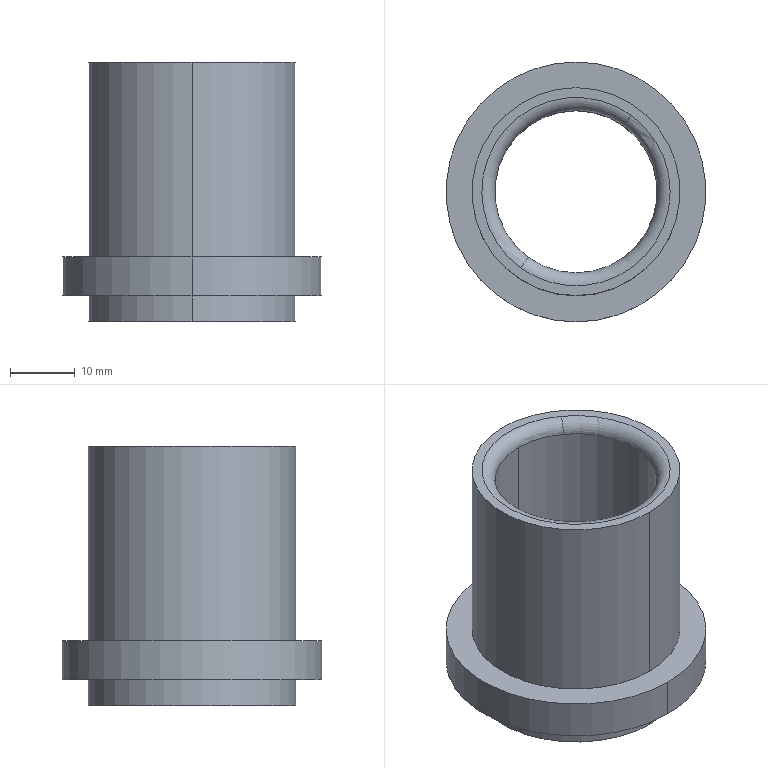Part | 1 solid | 16 faces | box 40 x 40 x 40 mm | volume 15162 mm3 | cylinder 8 | plane 4 | torus 4 | commonest cylinder face diameters 32 x4 25 x2 40 x2
STEP:
#1=CARTESIAN_POINT('',(0.,0.,0.));
#2=DIRECTION('',(0.,0.,1.));
#3=DIRECTION('',(1.,0.,0.));
#4=AXIS2_PLACEMENT_3D('',#1,#2,#3);
#5=CARTESIAN_POINT('',(-335.,26.5,-133.051));
#6=VERTEX_POINT('',#5);
#7=CARTESIAN_POINT('',(-335.,58.5,-133.051));
#8=VERTEX_POINT('',#7);
#9=CARTESIAN_POINT('',(-335.,42.5,-133.051));
#10=DIRECTION('',(0.,0.,1.));
#11=DIRECTION('',(0.,1.,0.));
#12=AXIS2_PLACEMENT_3D('',#9,#10,#11);
#13=CIRCLE('',#12,16.);
#14=CARTESIAN_POINT('',(-319.,42.5,-133.051));
#15=DIRECTION('',(0.,0.,-1.));
#16=DIRECTION('',(0.,-1.,0.));
#17=AXIS2_PLACEMENT_3D('',#14,#15,#16);
#18=PLANE('',#17);
#19=CARTESIAN_POINT('',(-16.,16.));
#20=CARTESIAN_POINT('',(-16.,43.713));
#21=CARTESIAN_POINT('',(8.,29.856));
#22=CARTESIAN_POINT('',(32.,16.));
#23=CARTESIAN_POINT('',(8.,2.144));
#24=CARTESIAN_POINT('',(-16.,-11.713));
#25=CARTESIAN_POINT('',(-16.,16.));
#26=(BOUNDED_CURVE()B_SPLINE_CURVE(2,(#19,#20,#21,#22,#23,#24,#25),.UNSPECIFIED.,.T.,.F.)B_SPLINE_CURVE_WITH_KNOTS((1,2,2,2,2,1),(-2.094,0.,2.094,4.189,6.283,8.378),.UNSPECIFIED.)CURVE()GEOMETRIC_REPRESENTATION_ITEM()RATIONAL_B_SPLINE_CURVE((1.,0.5,1.,0.5,1.,0.5,1.))REPRESENTATION_ITEM(''));
#27=(GEOMETRIC_REPRESENTATION_CONTEXT(2)PARAMETRIC_REPRESENTATION_CONTEXT()REPRESENTATION_CONTEXT('',''));
#28=DEFINITIONAL_REPRESENTATION('',(#26),#27);
#29=PCURVE('',#18,#28);
#30=CARTESIAN_POINT('',(-335.,42.5,-90.819));
#31=DIRECTION('',(0.,0.,1.));
#32=DIRECTION('',(-1.,0.,0.));
#33=AXIS2_PLACEMENT_3D('',#30,#31,#32);
#34=CYLINDRICAL_SURFACE('',#33,16.);
#35=CARTESIAN_POINT('',(-1.571,-42.232));
#36=DIRECTION('',(1.,0.));
#37=VECTOR('',#36,1.);
#38=LINE('',#35,#37);
#39=(GEOMETRIC_REPRESENTATION_CONTEXT(2)PARAMETRIC_REPRESENTATION_CONTEXT()REPRESENTATION_CONTEXT('',''));
#40=DEFINITIONAL_REPRESENTATION('',(#38),#39);
#41=PCURVE('',#34,#40);
#42=SURFACE_CURVE('',#13,(#29,#41),.PCURVE_S1.);
#43=EDGE_CURVE('',#6,#8,#42,.T.);
#44=ORIENTED_EDGE('',*,*,#43,.F.);
#45=CARTESIAN_POINT('',(-335.,42.5,-133.051));
#46=DIRECTION('',(0.,0.,1.));
#47=DIRECTION('',(0.,1.,0.));
#48=AXIS2_PLACEMENT_3D('',#45,#46,#47);
#49=CIRCLE('',#48,16.);
#50=CARTESIAN_POINT('',(-16.,16.));
#51=CARTESIAN_POINT('',(-16.,43.713));
#52=CARTESIAN_POINT('',(8.,29.856));
#53=CARTESIAN_POINT('',(32.,16.));
#54=CARTESIAN_POINT('',(8.,2.144));
#55=CARTESIAN_POINT('',(-16.,-11.713));
#56=CARTESIAN_POINT('',(-16.,16.));
#57=(BOUNDED_CURVE()B_SPLINE_CURVE(2,(#50,#51,#52,#53,#54,#55,#56),.UNSPECIFIED.,.T.,.F.)B_SPLINE_CURVE_WITH_KNOTS((1,2,2,2,2,1),(-2.094,0.,2.094,4.189,6.283,8.378),.UNSPECIFIED.)CURVE()GEOMETRIC_REPRESENTATION_ITEM()RATIONAL_B_SPLINE_CURVE((1.,0.5,1.,0.5,1.,0.5,1.))REPRESENTATION_ITEM(''));
#58=(GEOMETRIC_REPRESENTATION_CONTEXT(2)PARAMETRIC_REPRESENTATION_CONTEXT()REPRESENTATION_CONTEXT('',''));
#59=DEFINITIONAL_REPRESENTATION('',(#57),#58);
#60=PCURVE('',#18,#59);
#61=CARTESIAN_POINT('',(-335.,42.5,-90.819));
#62=DIRECTION('',(0.,0.,1.));
#63=DIRECTION('',(1.,0.,0.));
#64=AXIS2_PLACEMENT_3D('',#61,#62,#63);
#65=CYLINDRICAL_SURFACE('',#64,16.);
#66=CARTESIAN_POINT('',(1.571,-42.232));
#67=DIRECTION('',(1.,0.));
#68=VECTOR('',#67,1.);
#69=LINE('',#66,#68);
#70=(GEOMETRIC_REPRESENTATION_CONTEXT(2)PARAMETRIC_REPRESENTATION_CONTEXT()REPRESENTATION_CONTEXT('',''));
#71=DEFINITIONAL_REPRESENTATION('',(#69),#70);
#72=PCURVE('',#65,#71);
#73=SURFACE_CURVE('',#49,(#60,#72),.PCURVE_S1.);
#74=EDGE_CURVE('',#8,#6,#73,.T.);
#75=ORIENTED_EDGE('',*,*,#74,.F.);
#76=EDGE_LOOP('',(#44,#75));
#77=FACE_BOUND('',#76,.T.);
#78=CARTESIAN_POINT('',(-327.065,31.578,-133.051));
#79=VERTEX_POINT('',#78);
#80=CARTESIAN_POINT('',(-327.065,53.422,-133.051));
#81=VERTEX_POINT('',#80);
#82=CARTESIAN_POINT('',(-335.,42.5,-133.051));
#83=DIRECTION('',(0.,0.,1.));
#84=DIRECTION('',(0.5878,-0.809,0.));
#85=AXIS2_PLACEMENT_3D('',#82,#83,#84);
#86=CIRCLE('',#85,13.5);
#87=CARTESIAN_POINT('',(10.922,8.065));
#88=CARTESIAN_POINT('',(-2.822,-10.852));
#89=CARTESIAN_POINT('',(-12.333,10.509));
#90=CARTESIAN_POINT('',(-21.843,31.87));
#91=CARTESIAN_POINT('',(1.411,29.426));
#92=CARTESIAN_POINT('',(24.666,26.982));
#93=CARTESIAN_POINT('',(10.922,8.065));
#94=(BOUNDED_CURVE()B_SPLINE_CURVE(2,(#87,#88,#89,#90,#91,#92,#93),.UNSPECIFIED.,.T.,.F.)B_SPLINE_CURVE_WITH_KNOTS((1,2,2,2,2,1),(-2.094,0.,2.094,4.189,6.283,8.378),.UNSPECIFIED.)CURVE()GEOMETRIC_REPRESENTATION_ITEM()RATIONAL_B_SPLINE_CURVE((1.,0.5,1.,0.5,1.,0.5,1.))REPRESENTATION_ITEM(''));
#95=(GEOMETRIC_REPRESENTATION_CONTEXT(2)PARAMETRIC_REPRESENTATION_CONTEXT()REPRESENTATION_CONTEXT('',''));
#96=DEFINITIONAL_REPRESENTATION('',(#94),#95);
#97=PCURVE('',#18,#96);
#98=CARTESIAN_POINT('',(-335.,42.5,-132.051));
#99=DIRECTION('',(0.,0.,1.));
#100=DIRECTION('',(-0.809,0.5878,0.));
#101=AXIS2_PLACEMENT_3D('',#98,#99,#100);
#102=TOROIDAL_SURFACE('',#101,13.5,1.);
#103=CARTESIAN_POINT('',(2.827,4.712));
#104=DIRECTION('',(1.,0.));
#105=VECTOR('',#104,1.);
#106=LINE('',#103,#105);
#107=(GEOMETRIC_REPRESENTATION_CONTEXT(2)PARAMETRIC_REPRESENTATION_CONTEXT()REPRESENTATION_CONTEXT('',''));
#108=DEFINITIONAL_REPRESENTATION('',(#106),#107);
#109=PCURVE('',#102,#108);
#110=SURFACE_CURVE('',#86,(#97,#109),.PCURVE_S1.);
#111=EDGE_CURVE('',#79,#81,#110,.T.);
#112=ORIENTED_EDGE('',*,*,#111,.T.);
#113=CARTESIAN_POINT('',(-342.935,31.578,-133.051));
#114=VERTEX_POINT('',#113);
#115=CARTESIAN_POINT('',(-335.,42.5,-133.051));
#116=DIRECTION('',(0.,0.,1.));
#117=DIRECTION('',(0.5878,-0.809,0.));
#118=AXIS2_PLACEMENT_3D('',#115,#116,#117);
#119=CIRCLE('',#118,13.5);
#120=CARTESIAN_POINT('',(10.922,8.065));
#121=CARTESIAN_POINT('',(-2.822,-10.852));
#122=CARTESIAN_POINT('',(-12.333,10.509));
#123=CARTESIAN_POINT('',(-21.843,31.87));
#124=CARTESIAN_POINT('',(1.411,29.426));
#125=CARTESIAN_POINT('',(24.666,26.982));
#126=CARTESIAN_POINT('',(10.922,8.065));
#127=(BOUNDED_CURVE()B_SPLINE_CURVE(2,(#120,#121,#122,#123,#124,#125,#126),.UNSPECIFIED.,.T.,.F.)B_SPLINE_CURVE_WITH_KNOTS((1,2,2,2,2,1),(-2.094,0.,2.094,4.189,6.283,8.378),.UNSPECIFIED.)CURVE()GEOMETRIC_REPRESENTATION_ITEM()RATIONAL_B_SPLINE_CURVE((1.,0.5,1.,0.5,1.,0.5,1.))REPRESENTATION_ITEM(''));
#128=(GEOMETRIC_REPRESENTATION_CONTEXT(2)PARAMETRIC_REPRESENTATION_CONTEXT()REPRESENTATION_CONTEXT('',''));
#129=DEFINITIONAL_REPRESENTATION('',(#127),#128);
#130=PCURVE('',#18,#129);
#131=CARTESIAN_POINT('',(-335.,42.5,-132.051));
#132=DIRECTION('',(0.,0.,1.));
#133=DIRECTION('',(0.809,-0.5878,0.));
#134=AXIS2_PLACEMENT_3D('',#131,#132,#133);
#135=TOROIDAL_SURFACE('',#134,13.5,1.);
#136=CARTESIAN_POINT('',(-0.3142,4.712));
#137=DIRECTION('',(1.,0.));
#138=VECTOR('',#137,1.);
#139=LINE('',#136,#138);
#140=(GEOMETRIC_REPRESENTATION_CONTEXT(2)PARAMETRIC_REPRESENTATION_CONTEXT()REPRESENTATION_CONTEXT('',''));
#141=DEFINITIONAL_REPRESENTATION('',(#139),#140);
#142=PCURVE('',#135,#141);
#143=SURFACE_CURVE('',#119,(#130,#142),.PCURVE_S1.);
#144=EDGE_CURVE('',#81,#114,#143,.T.);
#145=ORIENTED_EDGE('',*,*,#144,.T.);
#146=CARTESIAN_POINT('',(-335.,42.5,-133.051));
#147=DIRECTION('',(0.,0.,1.));
#148=DIRECTION('',(0.5878,-0.809,0.));
#149=AXIS2_PLACEMENT_3D('',#146,#147,#148);
#150=CIRCLE('',#149,13.5);
#151=CARTESIAN_POINT('',(10.922,8.065));
#152=CARTESIAN_POINT('',(-2.822,-10.852));
#153=CARTESIAN_POINT('',(-12.333,10.509));
#154=CARTESIAN_POINT('',(-21.843,31.87));
#155=CARTESIAN_POINT('',(1.411,29.426));
#156=CARTESIAN_POINT('',(24.666,26.982));
#157=CARTESIAN_POINT('',(10.922,8.065));
#158=(BOUNDED_CURVE()B_SPLINE_CURVE(2,(#151,#152,#153,#154,#155,#156,#157),.UNSPECIFIED.,.T.,.F.)B_SPLINE_CURVE_WITH_KNOTS((1,2,2,2,2,1),(-2.094,0.,2.094,4.189,6.283,8.378),.UNSPECIFIED.)CURVE()GEOMETRIC_REPRESENTATION_ITEM()RATIONAL_B_SPLINE_CURVE((1.,0.5,1.,0.5,1.,0.5,1.))REPRESENTATION_ITEM(''));
#159=(GEOMETRIC_REPRESENTATION_CONTEXT(2)PARAMETRIC_REPRESENTATION_CONTEXT()REPRESENTATION_CONTEXT('',''));
#160=DEFINITIONAL_REPRESENTATION('',(#158),#159);
#161=PCURVE('',#18,#160);
#162=CARTESIAN_POINT('',(-3.456,4.712));
#163=DIRECTION('',(1.,0.));
#164=VECTOR('',#163,1.);
#165=LINE('',#162,#164);
#166=(GEOMETRIC_REPRESENTATION_CONTEXT(2)PARAMETRIC_REPRESENTATION_CONTEXT()REPRESENTATION_CONTEXT('',''));
#167=DEFINITIONAL_REPRESENTATION('',(#165),#166);
#168=PCURVE('',#102,#167);
#169=SURFACE_CURVE('',#150,(#161,#168),.PCURVE_S1.);
#170=EDGE_CURVE('',#114,#79,#169,.T.);
#171=ORIENTED_EDGE('',*,*,#170,.T.);
#172=EDGE_LOOP('',(#112,#145,#171));
#173=FACE_BOUND('',#172,.T.);
#174=ADVANCED_FACE('',(#77,#173),#18,.T.);
#175=CARTESIAN_POINT('',(-342.347,32.387,-132.051));
#176=VERTEX_POINT('',#175);
#177=CARTESIAN_POINT('',(-342.935,31.578,-132.051));
#178=DIRECTION('',(0.809,-0.5878,0.));
#179=DIRECTION('',(0.,0.,-1.));
#180=AXIS2_PLACEMENT_3D('',#177,#178,#179);
#181=CIRCLE('',#180,1.);
#182=CARTESIAN_POINT('',(1.571,4.712));
#183=DIRECTION('',(0.,-1.));
#184=VECTOR('',#183,1.);
#185=LINE('',#182,#184);
#186=(GEOMETRIC_REPRESENTATION_CONTEXT(2)PARAMETRIC_REPRESENTATION_CONTEXT()REPRESENTATION_CONTEXT('',''));
#187=DEFINITIONAL_REPRESENTATION('',(#185),#186);
#188=PCURVE('',#102,#187);
#189=CARTESIAN_POINT('',(4.712,4.712));
#190=DIRECTION('',(0.,-1.));
#191=VECTOR('',#190,1.);
#192=LINE('',#189,#191);
#193=(GEOMETRIC_REPRESENTATION_CONTEXT(2)PARAMETRIC_REPRESENTATION_CONTEXT()REPRESENTATION_CONTEXT('',''));
#194=DEFINITIONAL_REPRESENTATION('',(#192),#193);
#195=PCURVE('',#135,#194);
#196=SURFACE_CURVE('',#181,(#188,#195),.PCURVE_S1.);
#197=EDGE_CURVE('',#114,#176,#196,.T.);
#198=ORIENTED_EDGE('',*,*,#197,.T.);
#199=CARTESIAN_POINT('',(-335.,30.,-132.051));
#200=VERTEX_POINT('',#199);
#201=CARTESIAN_POINT('',(-335.,42.5,-132.051));
#202=DIRECTION('',(0.,0.,-1.));
#203=DIRECTION('',(0.5878,-0.809,0.));
#204=AXIS2_PLACEMENT_3D('',#201,#202,#203);
#205=CIRCLE('',#204,12.5);
#206=CARTESIAN_POINT('',(2.827,3.142));
#207=DIRECTION('',(-1.,0.));
#208=VECTOR('',#207,1.);
#209=LINE('',#206,#208);
#210=(GEOMETRIC_REPRESENTATION_CONTEXT(2)PARAMETRIC_REPRESENTATION_CONTEXT()REPRESENTATION_CONTEXT('',''));
#211=DEFINITIONAL_REPRESENTATION('',(#209),#210);
#212=PCURVE('',#102,#211);
#213=CARTESIAN_POINT('',(-335.,42.5,-90.819));
#214=DIRECTION('',(0.,0.,1.));
#215=DIRECTION('',(1.,0.,0.));
#216=AXIS2_PLACEMENT_3D('',#213,#214,#215);
#217=CYLINDRICAL_SURFACE('',#216,12.5);
#218=CARTESIAN_POINT('',(5.341,-41.232));
#219=DIRECTION('',(-1.,0.));
#220=VECTOR('',#219,1.);
#221=LINE('',#218,#220);
#222=(GEOMETRIC_REPRESENTATION_CONTEXT(2)PARAMETRIC_REPRESENTATION_CONTEXT()REPRESENTATION_CONTEXT('',''));
#223=DEFINITIONAL_REPRESENTATION('',(#221),#222);
#224=PCURVE('',#217,#223);
#225=SURFACE_CURVE('',#205,(#212,#224),.PCURVE_S1.);
#226=EDGE_CURVE('',#200,#176,#225,.T.);
#227=ORIENTED_EDGE('',*,*,#226,.F.);
#228=CARTESIAN_POINT('',(-327.652,32.387,-132.051));
#229=VERTEX_POINT('',#228);
#230=CARTESIAN_POINT('',(-335.,42.5,-132.051));
#231=DIRECTION('',(0.,0.,-1.));
#232=DIRECTION('',(0.5878,-0.809,0.));
#233=AXIS2_PLACEMENT_3D('',#230,#231,#232);
#234=CIRCLE('',#233,12.5);
#235=CARTESIAN_POINT('',(2.827,3.142));
#236=DIRECTION('',(-1.,0.));
#237=VECTOR('',#236,1.);
#238=LINE('',#235,#237);
#239=(GEOMETRIC_REPRESENTATION_CONTEXT(2)PARAMETRIC_REPRESENTATION_CONTEXT()REPRESENTATION_CONTEXT('',''));
#240=DEFINITIONAL_REPRESENTATION('',(#238),#239);
#241=PCURVE('',#102,#240);
#242=CARTESIAN_POINT('',(-335.,42.5,-90.819));
#243=DIRECTION('',(0.,0.,1.));
#244=DIRECTION('',(-1.,0.,0.));
#245=AXIS2_PLACEMENT_3D('',#242,#243,#244);
#246=CYLINDRICAL_SURFACE('',#245,12.5);
#247=CARTESIAN_POINT('',(2.199,-41.232));
#248=DIRECTION('',(-1.,0.));
#249=VECTOR('',#248,1.);
#250=LINE('',#247,#249);
#251=(GEOMETRIC_REPRESENTATION_CONTEXT(2)PARAMETRIC_REPRESENTATION_CONTEXT()REPRESENTATION_CONTEXT('',''));
#252=DEFINITIONAL_REPRESENTATION('',(#250),#251);
#253=PCURVE('',#246,#252);
#254=SURFACE_CURVE('',#234,(#241,#253),.PCURVE_S1.);
#255=EDGE_CURVE('',#229,#200,#254,.T.);
#256=ORIENTED_EDGE('',*,*,#255,.F.);
#257=CARTESIAN_POINT('',(-327.652,52.613,-132.051));
#258=VERTEX_POINT('',#257);
#259=CARTESIAN_POINT('',(-335.,42.5,-132.051));
#260=DIRECTION('',(0.,0.,-1.));
#261=DIRECTION('',(0.5878,-0.809,0.));
#262=AXIS2_PLACEMENT_3D('',#259,#260,#261);
#263=CIRCLE('',#262,12.5);
#264=CARTESIAN_POINT('',(9.111,3.142));
#265=DIRECTION('',(-1.,0.));
#266=VECTOR('',#265,1.);
#267=LINE('',#264,#266);
#268=(GEOMETRIC_REPRESENTATION_CONTEXT(2)PARAMETRIC_REPRESENTATION_CONTEXT()REPRESENTATION_CONTEXT('',''));
#269=DEFINITIONAL_REPRESENTATION('',(#267),#268);
#270=PCURVE('',#102,#269);
#271=CARTESIAN_POINT('',(8.482,-41.232));
#272=DIRECTION('',(-1.,0.));
#273=VECTOR('',#272,1.);
#274=LINE('',#271,#273);
#275=(GEOMETRIC_REPRESENTATION_CONTEXT(2)PARAMETRIC_REPRESENTATION_CONTEXT()REPRESENTATION_CONTEXT('',''));
#276=DEFINITIONAL_REPRESENTATION('',(#274),#275);
#277=PCURVE('',#246,#276);
#278=SURFACE_CURVE('',#263,(#270,#277),.PCURVE_S1.);
#279=EDGE_CURVE('',#258,#229,#278,.T.);
#280=ORIENTED_EDGE('',*,*,#279,.F.);
#281=CARTESIAN_POINT('',(-327.065,53.422,-132.051));
#282=DIRECTION('',(-0.809,0.5878,0.));
#283=DIRECTION('',(0.,0.,-1.));
#284=AXIS2_PLACEMENT_3D('',#281,#282,#283);
#285=CIRCLE('',#284,1.);
#286=CARTESIAN_POINT('',(4.712,4.712));
#287=DIRECTION('',(0.,-1.));
#288=VECTOR('',#287,1.);
#289=LINE('',#286,#288);
#290=(GEOMETRIC_REPRESENTATION_CONTEXT(2)PARAMETRIC_REPRESENTATION_CONTEXT()REPRESENTATION_CONTEXT('',''));
#291=DEFINITIONAL_REPRESENTATION('',(#289),#290);
#292=PCURVE('',#102,#291);
#293=CARTESIAN_POINT('',(1.571,4.712));
#294=DIRECTION('',(0.,-1.));
#295=VECTOR('',#294,1.);
#296=LINE('',#293,#295);
#297=(GEOMETRIC_REPRESENTATION_CONTEXT(2)PARAMETRIC_REPRESENTATION_CONTEXT()REPRESENTATION_CONTEXT('',''));
#298=DEFINITIONAL_REPRESENTATION('',(#296),#297);
#299=PCURVE('',#135,#298);
#300=SURFACE_CURVE('',#285,(#292,#299),.PCURVE_S1.);
#301=EDGE_CURVE('',#81,#258,#300,.T.);
#302=ORIENTED_EDGE('',*,*,#301,.F.);
#303=ORIENTED_EDGE('',*,*,#111,.F.);
#304=ORIENTED_EDGE('',*,*,#170,.F.);
#305=EDGE_LOOP('',(#198,#227,#256,#280,#302,#303,#304));
#306=FACE_BOUND('',#305,.T.);
#307=ADVANCED_FACE('',(#306),#102,.T.);
#308=ORIENTED_EDGE('',*,*,#255,.F.);
#309=ORIENTED_EDGE('',*,*,#279,.F.);
#310=CARTESIAN_POINT('',(-335.,55.,-132.051));
#311=VERTEX_POINT('',#310);
#312=CARTESIAN_POINT('',(-335.,42.5,-132.051));
#313=DIRECTION('',(0.,0.,-1.));
#314=DIRECTION('',(0.5878,-0.809,0.));
#315=AXIS2_PLACEMENT_3D('',#312,#313,#314);
#316=CIRCLE('',#315,12.5);
#317=CARTESIAN_POINT('',(8.482,-41.232));
#318=DIRECTION('',(-1.,0.));
#319=VECTOR('',#318,1.);
#320=LINE('',#317,#319);
#321=(GEOMETRIC_REPRESENTATION_CONTEXT(2)PARAMETRIC_REPRESENTATION_CONTEXT()REPRESENTATION_CONTEXT('',''));
#322=DEFINITIONAL_REPRESENTATION('',(#320),#321);
#323=PCURVE('',#246,#322);
#324=CARTESIAN_POINT('',(5.969,3.142));
#325=DIRECTION('',(-1.,0.));
#326=VECTOR('',#325,1.);
#327=LINE('',#324,#326);
#328=(GEOMETRIC_REPRESENTATION_CONTEXT(2)PARAMETRIC_REPRESENTATION_CONTEXT()REPRESENTATION_CONTEXT('',''));
#329=DEFINITIONAL_REPRESENTATION('',(#327),#328);
#330=PCURVE('',#135,#329);
#331=SURFACE_CURVE('',#316,(#323,#330),.PCURVE_S1.);
#332=EDGE_CURVE('',#311,#258,#331,.T.);
#333=ORIENTED_EDGE('',*,*,#332,.F.);
#334=CARTESIAN_POINT('',(-335.,55.,-95.051));
#335=VERTEX_POINT('',#334);
#336=CARTESIAN_POINT('',(-335.,55.,-132.051));
#337=DIRECTION('',(0.,0.,1.));
#338=VECTOR('',#337,1.);
#339=LINE('',#336,#338);
#340=CARTESIAN_POINT('',(4.712,-41.232));
#341=DIRECTION('',(0.,1.));
#342=VECTOR('',#341,1.);
#343=LINE('',#340,#342);
#344=(GEOMETRIC_REPRESENTATION_CONTEXT(2)PARAMETRIC_REPRESENTATION_CONTEXT()REPRESENTATION_CONTEXT('',''));
#345=DEFINITIONAL_REPRESENTATION('',(#343),#344);
#346=PCURVE('',#246,#345);
#347=CARTESIAN_POINT('',(1.571,-41.232));
#348=DIRECTION('',(0.,1.));
#349=VECTOR('',#348,1.);
#350=LINE('',#347,#349);
#351=(GEOMETRIC_REPRESENTATION_CONTEXT(2)PARAMETRIC_REPRESENTATION_CONTEXT()REPRESENTATION_CONTEXT('',''));
#352=DEFINITIONAL_REPRESENTATION('',(#350),#351);
#353=PCURVE('',#217,#352);
#354=SURFACE_CURVE('',#339,(#346,#353),.PCURVE_S1.);
#355=EDGE_CURVE('',#311,#335,#354,.T.);
#356=ORIENTED_EDGE('',*,*,#355,.T.);
#357=CARTESIAN_POINT('',(-327.652,52.613,-95.051));
#358=VERTEX_POINT('',#357);
#359=CARTESIAN_POINT('',(-335.,42.5,-95.051));
#360=DIRECTION('',(0.,0.,-1.));
#361=DIRECTION('',(0.,-1.,0.));
#362=AXIS2_PLACEMENT_3D('',#359,#360,#361);
#363=CIRCLE('',#362,12.5);
#364=CARTESIAN_POINT('',(7.854,-4.232));
#365=DIRECTION('',(-1.,0.));
#366=VECTOR('',#365,1.);
#367=LINE('',#364,#366);
#368=(GEOMETRIC_REPRESENTATION_CONTEXT(2)PARAMETRIC_REPRESENTATION_CONTEXT()REPRESENTATION_CONTEXT('',''));
#369=DEFINITIONAL_REPRESENTATION('',(#367),#368);
#370=PCURVE('',#246,#369);
#371=CARTESIAN_POINT('',(-335.,42.5,-95.051));
#372=DIRECTION('',(0.,0.,1.));
#373=DIRECTION('',(0.809,-0.5878,0.));
#374=AXIS2_PLACEMENT_3D('',#371,#372,#373);
#375=TOROIDAL_SURFACE('',#374,14.5,2.);
#376=CARTESIAN_POINT('',(5.341,3.142));
#377=DIRECTION('',(-1.,0.));
#378=VECTOR('',#377,1.);
#379=LINE('',#376,#378);
#380=(GEOMETRIC_REPRESENTATION_CONTEXT(2)PARAMETRIC_REPRESENTATION_CONTEXT()REPRESENTATION_CONTEXT('',''));
#381=DEFINITIONAL_REPRESENTATION('',(#379),#380);
#382=PCURVE('',#375,#381);
#383=SURFACE_CURVE('',#363,(#370,#382),.PCURVE_S1.);
#384=EDGE_CURVE('',#335,#358,#383,.T.);
#385=ORIENTED_EDGE('',*,*,#384,.T.);
#386=CARTESIAN_POINT('',(-335.,30.,-95.051));
#387=VERTEX_POINT('',#386);
#388=CARTESIAN_POINT('',(-335.,42.5,-95.051));
#389=DIRECTION('',(0.,0.,-1.));
#390=DIRECTION('',(0.,-1.,0.));
#391=AXIS2_PLACEMENT_3D('',#388,#389,#390);
#392=CIRCLE('',#391,12.5);
#393=CARTESIAN_POINT('',(7.854,-4.232));
#394=DIRECTION('',(-1.,0.));
#395=VECTOR('',#394,1.);
#396=LINE('',#393,#395);
#397=(GEOMETRIC_REPRESENTATION_CONTEXT(2)PARAMETRIC_REPRESENTATION_CONTEXT()REPRESENTATION_CONTEXT('',''));
#398=DEFINITIONAL_REPRESENTATION('',(#396),#397);
#399=PCURVE('',#246,#398);
#400=CARTESIAN_POINT('',(-335.,42.5,-95.051));
#401=DIRECTION('',(0.,0.,1.));
#402=DIRECTION('',(-0.809,0.5878,0.));
#403=AXIS2_PLACEMENT_3D('',#400,#401,#402);
#404=TOROIDAL_SURFACE('',#403,14.5,2.);
#405=CARTESIAN_POINT('',(8.482,3.142));
#406=DIRECTION('',(-1.,0.));
#407=VECTOR('',#406,1.);
#408=LINE('',#405,#407);
#409=(GEOMETRIC_REPRESENTATION_CONTEXT(2)PARAMETRIC_REPRESENTATION_CONTEXT()REPRESENTATION_CONTEXT('',''));
#410=DEFINITIONAL_REPRESENTATION('',(#408),#409);
#411=PCURVE('',#404,#410);
#412=SURFACE_CURVE('',#392,(#399,#411),.PCURVE_S1.);
#413=EDGE_CURVE('',#358,#387,#412,.T.);
#414=ORIENTED_EDGE('',*,*,#413,.T.);
#415=CARTESIAN_POINT('',(-335.,30.,-132.051));
#416=DIRECTION('',(0.,0.,1.));
#417=VECTOR('',#416,1.);
#418=LINE('',#415,#417);
#419=CARTESIAN_POINT('',(1.571,-41.232));
#420=DIRECTION('',(0.,1.));
#421=VECTOR('',#420,1.);
#422=LINE('',#419,#421);
#423=(GEOMETRIC_REPRESENTATION_CONTEXT(2)PARAMETRIC_REPRESENTATION_CONTEXT()REPRESENTATION_CONTEXT('',''));
#424=DEFINITIONAL_REPRESENTATION('',(#422),#423);
#425=PCURVE('',#246,#424);
#426=CARTESIAN_POINT('',(4.712,-41.232));
#427=DIRECTION('',(0.,1.));
#428=VECTOR('',#427,1.);
#429=LINE('',#426,#428);
#430=(GEOMETRIC_REPRESENTATION_CONTEXT(2)PARAMETRIC_REPRESENTATION_CONTEXT()REPRESENTATION_CONTEXT('',''));
#431=DEFINITIONAL_REPRESENTATION('',(#429),#430);
#432=PCURVE('',#217,#431);
#433=SURFACE_CURVE('',#418,(#425,#432),.PCURVE_S1.);
#434=EDGE_CURVE('',#200,#387,#433,.T.);
#435=ORIENTED_EDGE('',*,*,#434,.F.);
#436=EDGE_LOOP('',(#308,#309,#333,#356,#385,#414,#435));
#437=FACE_BOUND('',#436,.F.);
#438=ADVANCED_FACE('',(#437),#246,.F.);
#439=CARTESIAN_POINT('',(-342.347,32.387,-95.051));
#440=VERTEX_POINT('',#439);
#441=CARTESIAN_POINT('',(-343.523,30.769,-93.051));
#442=VERTEX_POINT('',#441);
#443=CARTESIAN_POINT('',(-343.523,30.769,-95.051));
#444=DIRECTION('',(0.809,-0.5878,0.));
#445=DIRECTION('',(0.5878,0.809,0.));
#446=AXIS2_PLACEMENT_3D('',#443,#444,#445);
#447=CIRCLE('',#446,2.);
#448=CARTESIAN_POINT('',(1.571,3.142));
#449=DIRECTION('',(0.,-1.));
#450=VECTOR('',#449,1.);
#451=LINE('',#448,#450);
#452=(GEOMETRIC_REPRESENTATION_CONTEXT(2)PARAMETRIC_REPRESENTATION_CONTEXT()REPRESENTATION_CONTEXT('',''));
#453=DEFINITIONAL_REPRESENTATION('',(#451),#452);
#454=PCURVE('',#404,#453);
#455=CARTESIAN_POINT('',(4.712,3.142));
#456=DIRECTION('',(0.,-1.));
#457=VECTOR('',#456,1.);
#458=LINE('',#455,#457);
#459=(GEOMETRIC_REPRESENTATION_CONTEXT(2)PARAMETRIC_REPRESENTATION_CONTEXT()REPRESENTATION_CONTEXT('',''));
#460=DEFINITIONAL_REPRESENTATION('',(#458),#459);
#461=PCURVE('',#375,#460);
#462=SURFACE_CURVE('',#447,(#454,#461),.PCURVE_S1.);
#463=EDGE_CURVE('',#440,#442,#462,.T.);
#464=ORIENTED_EDGE('',*,*,#463,.T.);
#465=CARTESIAN_POINT('',(-326.477,30.769,-93.051));
#466=VERTEX_POINT('',#465);
#467=CARTESIAN_POINT('',(-335.,42.5,-93.051));
#468=DIRECTION('',(0.,0.,1.));
#469=DIRECTION('',(0.5878,-0.809,0.));
#470=AXIS2_PLACEMENT_3D('',#467,#468,#469);
#471=CIRCLE('',#470,14.5);
#472=CARTESIAN_POINT('',(-3.456,1.571));
#473=DIRECTION('',(1.,0.));
#474=VECTOR('',#473,1.);
#475=LINE('',#472,#474);
#476=(GEOMETRIC_REPRESENTATION_CONTEXT(2)PARAMETRIC_REPRESENTATION_CONTEXT()REPRESENTATION_CONTEXT('',''));
#477=DEFINITIONAL_REPRESENTATION('',(#475),#476);
#478=PCURVE('',#404,#477);
#479=CARTESIAN_POINT('',(-335.,42.5,-93.051));
#480=DIRECTION('',(0.,0.,1.));
#481=DIRECTION('',(0.,1.,0.));
#482=AXIS2_PLACEMENT_3D('',#479,#480,#481);
#483=PLANE('',#482);
#484=CARTESIAN_POINT('',(0.,0.));
#485=DIRECTION('',(-0.809,-0.5878));
#486=AXIS2_PLACEMENT_2D('',#484,#485);
#487=CIRCLE('',#486,14.5);
#488=(GEOMETRIC_REPRESENTATION_CONTEXT(2)PARAMETRIC_REPRESENTATION_CONTEXT()REPRESENTATION_CONTEXT('',''));
#489=DEFINITIONAL_REPRESENTATION('',(#487),#488);
#490=PCURVE('',#483,#489);
#491=SURFACE_CURVE('',#471,(#478,#490),.PCURVE_S1.);
#492=EDGE_CURVE('',#442,#466,#491,.T.);
#493=ORIENTED_EDGE('',*,*,#492,.T.);
#494=CARTESIAN_POINT('',(-326.477,54.231,-93.051));
#495=VERTEX_POINT('',#494);
#496=CARTESIAN_POINT('',(-335.,42.5,-93.051));
#497=DIRECTION('',(0.,0.,1.));
#498=DIRECTION('',(0.5878,-0.809,0.));
#499=AXIS2_PLACEMENT_3D('',#496,#497,#498);
#500=CIRCLE('',#499,14.5);
#501=CARTESIAN_POINT('',(2.827,1.571));
#502=DIRECTION('',(1.,0.));
#503=VECTOR('',#502,1.);
#504=LINE('',#501,#503);
#505=(GEOMETRIC_REPRESENTATION_CONTEXT(2)PARAMETRIC_REPRESENTATION_CONTEXT()REPRESENTATION_CONTEXT('',''));
#506=DEFINITIONAL_REPRESENTATION('',(#504),#505);
#507=PCURVE('',#404,#506);
#508=CARTESIAN_POINT('',(0.,0.));
#509=DIRECTION('',(-0.809,-0.5878));
#510=AXIS2_PLACEMENT_2D('',#508,#509);
#511=CIRCLE('',#510,14.5);
#512=(GEOMETRIC_REPRESENTATION_CONTEXT(2)PARAMETRIC_REPRESENTATION_CONTEXT()REPRESENTATION_CONTEXT('',''));
#513=DEFINITIONAL_REPRESENTATION('',(#511),#512);
#514=PCURVE('',#483,#513);
#515=SURFACE_CURVE('',#500,(#507,#514),.PCURVE_S1.);
#516=EDGE_CURVE('',#466,#495,#515,.T.);
#517=ORIENTED_EDGE('',*,*,#516,.T.);
#518=CARTESIAN_POINT('',(-326.477,54.231,-95.051));
#519=DIRECTION('',(-0.809,0.5878,0.));
#520=DIRECTION('',(-0.5878,-0.809,0.));
#521=AXIS2_PLACEMENT_3D('',#518,#519,#520);
#522=CIRCLE('',#521,2.);
#523=CARTESIAN_POINT('',(4.712,3.142));
#524=DIRECTION('',(0.,-1.));
#525=VECTOR('',#524,1.);
#526=LINE('',#523,#525);
#527=(GEOMETRIC_REPRESENTATION_CONTEXT(2)PARAMETRIC_REPRESENTATION_CONTEXT()REPRESENTATION_CONTEXT('',''));
#528=DEFINITIONAL_REPRESENTATION('',(#526),#527);
#529=PCURVE('',#404,#528);
#530=CARTESIAN_POINT('',(1.571,3.142));
#531=DIRECTION('',(0.,-1.));
#532=VECTOR('',#531,1.);
#533=LINE('',#530,#532);
#534=(GEOMETRIC_REPRESENTATION_CONTEXT(2)PARAMETRIC_REPRESENTATION_CONTEXT()REPRESENTATION_CONTEXT('',''));
#535=DEFINITIONAL_REPRESENTATION('',(#533),#534);
#536=PCURVE('',#375,#535);
#537=SURFACE_CURVE('',#522,(#529,#536),.PCURVE_S1.);
#538=EDGE_CURVE('',#358,#495,#537,.T.);
#539=ORIENTED_EDGE('',*,*,#538,.F.);
#540=ORIENTED_EDGE('',*,*,#413,.T.);
#541=CARTESIAN_POINT('',(-335.,42.5,-95.051));
#542=DIRECTION('',(0.,0.,-1.));
#543=DIRECTION('',(0.,-1.,0.));
#544=AXIS2_PLACEMENT_3D('',#541,#542,#543);
#545=CIRCLE('',#544,12.5);
#546=CARTESIAN_POINT('',(2.199,3.142));
#547=DIRECTION('',(-1.,0.));
#548=VECTOR('',#547,1.);
#549=LINE('',#546,#548);
#550=(GEOMETRIC_REPRESENTATION_CONTEXT(2)PARAMETRIC_REPRESENTATION_CONTEXT()REPRESENTATION_CONTEXT('',''));
#551=DEFINITIONAL_REPRESENTATION('',(#549),#550);
#552=PCURVE('',#404,#551);
#553=CARTESIAN_POINT('',(4.712,-4.232));
#554=DIRECTION('',(-1.,0.));
#555=VECTOR('',#554,1.);
#556=LINE('',#553,#555);
#557=(GEOMETRIC_REPRESENTATION_CONTEXT(2)PARAMETRIC_REPRESENTATION_CONTEXT()REPRESENTATION_CONTEXT('',''));
#558=DEFINITIONAL_REPRESENTATION('',(#556),#557);
#559=PCURVE('',#217,#558);
#560=SURFACE_CURVE('',#545,(#552,#559),.PCURVE_S1.);
#561=EDGE_CURVE('',#387,#440,#560,.T.);
#562=ORIENTED_EDGE('',*,*,#561,.T.);
#563=EDGE_LOOP('',(#464,#493,#517,#539,#540,#562));
#564=FACE_BOUND('',#563,.T.);
#565=ADVANCED_FACE('',(#564),#404,.T.);
#566=ORIENTED_EDGE('',*,*,#492,.F.);
#567=CARTESIAN_POINT('',(-335.,42.5,-93.051));
#568=DIRECTION('',(0.,0.,1.));
#569=DIRECTION('',(0.5878,-0.809,0.));
#570=AXIS2_PLACEMENT_3D('',#567,#568,#569);
#571=CIRCLE('',#570,14.5);
#572=CARTESIAN_POINT('',(0.,0.));
#573=DIRECTION('',(-0.809,-0.5878));
#574=AXIS2_PLACEMENT_2D('',#572,#573);
#575=CIRCLE('',#574,14.5);
#576=(GEOMETRIC_REPRESENTATION_CONTEXT(2)PARAMETRIC_REPRESENTATION_CONTEXT()REPRESENTATION_CONTEXT('',''));
#577=DEFINITIONAL_REPRESENTATION('',(#575),#576);
#578=PCURVE('',#483,#577);
#579=CARTESIAN_POINT('',(-0.3142,1.571));
#580=DIRECTION('',(1.,0.));
#581=VECTOR('',#580,1.);
#582=LINE('',#579,#581);
#583=(GEOMETRIC_REPRESENTATION_CONTEXT(2)PARAMETRIC_REPRESENTATION_CONTEXT()REPRESENTATION_CONTEXT('',''));
#584=DEFINITIONAL_REPRESENTATION('',(#582),#583);
#585=PCURVE('',#375,#584);
#586=SURFACE_CURVE('',#571,(#578,#585),.PCURVE_S1.);
#587=EDGE_CURVE('',#495,#442,#586,.T.);
#588=ORIENTED_EDGE('',*,*,#587,.F.);
#589=ORIENTED_EDGE('',*,*,#516,.F.);
#590=EDGE_LOOP('',(#566,#588,#589));
#591=FACE_BOUND('',#590,.T.);
#592=CARTESIAN_POINT('',(-335.,58.5,-93.051));
#593=VERTEX_POINT('',#592);
#594=CARTESIAN_POINT('',(-335.,26.5,-93.051));
#595=VERTEX_POINT('',#594);
#596=CARTESIAN_POINT('',(-335.,42.5,-93.051));
#597=DIRECTION('',(0.,0.,1.));
#598=DIRECTION('',(0.,1.,0.));
#599=AXIS2_PLACEMENT_3D('',#596,#597,#598);
#600=CIRCLE('',#599,16.);
#601=CARTESIAN_POINT('',(0.,0.));
#602=DIRECTION('',(1.,0.));
#603=AXIS2_PLACEMENT_2D('',#601,#602);
#604=CIRCLE('',#603,16.);
#605=(GEOMETRIC_REPRESENTATION_CONTEXT(2)PARAMETRIC_REPRESENTATION_CONTEXT()REPRESENTATION_CONTEXT('',''));
#606=DEFINITIONAL_REPRESENTATION('',(#604),#605);
#607=PCURVE('',#483,#606);
#608=CARTESIAN_POINT('',(-335.,42.5,-90.819));
#609=DIRECTION('',(0.,0.,1.));
#610=DIRECTION('',(1.,0.,0.));
#611=AXIS2_PLACEMENT_3D('',#608,#609,#610);
#612=CYLINDRICAL_SURFACE('',#611,16.);
#613=CARTESIAN_POINT('',(1.571,-2.232));
#614=DIRECTION('',(1.,0.));
#615=VECTOR('',#614,1.);
#616=LINE('',#613,#615);
#617=(GEOMETRIC_REPRESENTATION_CONTEXT(2)PARAMETRIC_REPRESENTATION_CONTEXT()REPRESENTATION_CONTEXT('',''));
#618=DEFINITIONAL_REPRESENTATION('',(#616),#617);
#619=PCURVE('',#612,#618);
#620=SURFACE_CURVE('',#600,(#607,#619),.PCURVE_S1.);
#621=EDGE_CURVE('',#593,#595,#620,.T.);
#622=ORIENTED_EDGE('',*,*,#621,.T.);
#623=CARTESIAN_POINT('',(-335.,42.5,-93.051));
#624=DIRECTION('',(0.,0.,1.));
#625=DIRECTION('',(0.,1.,0.));
#626=AXIS2_PLACEMENT_3D('',#623,#624,#625);
#627=CIRCLE('',#626,16.);
#628=CARTESIAN_POINT('',(0.,0.));
#629=DIRECTION('',(1.,0.));
#630=AXIS2_PLACEMENT_2D('',#628,#629);
#631=CIRCLE('',#630,16.);
#632=(GEOMETRIC_REPRESENTATION_CONTEXT(2)PARAMETRIC_REPRESENTATION_CONTEXT()REPRESENTATION_CONTEXT('',''));
#633=DEFINITIONAL_REPRESENTATION('',(#631),#632);
#634=PCURVE('',#483,#633);
#635=CARTESIAN_POINT('',(-335.,42.5,-90.819));
#636=DIRECTION('',(0.,0.,1.));
#637=DIRECTION('',(-1.,0.,0.));
#638=AXIS2_PLACEMENT_3D('',#635,#636,#637);
#639=CYLINDRICAL_SURFACE('',#638,16.);
#640=CARTESIAN_POINT('',(-1.571,-2.232));
#641=DIRECTION('',(1.,0.));
#642=VECTOR('',#641,1.);
#643=LINE('',#640,#642);
#644=(GEOMETRIC_REPRESENTATION_CONTEXT(2)PARAMETRIC_REPRESENTATION_CONTEXT()REPRESENTATION_CONTEXT('',''));
#645=DEFINITIONAL_REPRESENTATION('',(#643),#644);
#646=PCURVE('',#639,#645);
#647=SURFACE_CURVE('',#627,(#634,#646),.PCURVE_S1.);
#648=EDGE_CURVE('',#595,#593,#647,.T.);
#649=ORIENTED_EDGE('',*,*,#648,.T.);
#650=EDGE_LOOP('',(#622,#649));
#651=FACE_BOUND('',#650,.T.);
#652=ADVANCED_FACE('',(#591,#651),#483,.T.);
#653=CARTESIAN_POINT('',(-335.,26.5,-123.051));
#654=VERTEX_POINT('',#653);
#655=CARTESIAN_POINT('',(-335.,26.5,-123.051));
#656=DIRECTION('',(0.,0.,1.));
#657=VECTOR('',#656,1.);
#658=LINE('',#655,#657);
#659=CARTESIAN_POINT('',(1.571,-32.232));
#660=DIRECTION('',(0.,1.));
#661=VECTOR('',#660,1.);
#662=LINE('',#659,#661);
#663=(GEOMETRIC_REPRESENTATION_CONTEXT(2)PARAMETRIC_REPRESENTATION_CONTEXT()REPRESENTATION_CONTEXT('',''));
#664=DEFINITIONAL_REPRESENTATION('',(#662),#663);
#665=PCURVE('',#639,#664);
#666=CARTESIAN_POINT('',(4.712,-32.232));
#667=DIRECTION('',(0.,1.));
#668=VECTOR('',#667,1.);
#669=LINE('',#666,#668);
#670=(GEOMETRIC_REPRESENTATION_CONTEXT(2)PARAMETRIC_REPRESENTATION_CONTEXT()REPRESENTATION_CONTEXT('',''));
#671=DEFINITIONAL_REPRESENTATION('',(#669),#670);
#672=PCURVE('',#612,#671);
#673=SURFACE_CURVE('',#658,(#665,#672),.PCURVE_S1.);
#674=EDGE_CURVE('',#654,#595,#673,.T.);
#675=ORIENTED_EDGE('',*,*,#674,.F.);
#676=CARTESIAN_POINT('',(-335.,58.5,-123.051));
#677=VERTEX_POINT('',#676);
#678=CARTESIAN_POINT('',(-335.,42.5,-123.051));
#679=DIRECTION('',(0.,0.,1.));
#680=DIRECTION('',(0.,1.,0.));
#681=AXIS2_PLACEMENT_3D('',#678,#679,#680);
#682=CIRCLE('',#681,16.);
#683=CARTESIAN_POINT('',(-1.571,-32.232));
#684=DIRECTION('',(1.,0.));
#685=VECTOR('',#684,1.);
#686=LINE('',#683,#685);
#687=(GEOMETRIC_REPRESENTATION_CONTEXT(2)PARAMETRIC_REPRESENTATION_CONTEXT()REPRESENTATION_CONTEXT('',''));
#688=DEFINITIONAL_REPRESENTATION('',(#686),#687);
#689=PCURVE('',#639,#688);
#690=CARTESIAN_POINT('',(-319.,42.5,-123.051));
#691=DIRECTION('',(0.,0.,1.));
#692=DIRECTION('',(0.,1.,0.));
#693=AXIS2_PLACEMENT_3D('',#690,#691,#692);
#694=PLANE('',#693);
#695=CARTESIAN_POINT('',(0.,16.));
#696=DIRECTION('',(1.,0.));
#697=AXIS2_PLACEMENT_2D('',#695,#696);
#698=CIRCLE('',#697,16.);
#699=(GEOMETRIC_REPRESENTATION_CONTEXT(2)PARAMETRIC_REPRESENTATION_CONTEXT()REPRESENTATION_CONTEXT('',''));
#700=DEFINITIONAL_REPRESENTATION('',(#698),#699);
#701=PCURVE('',#694,#700);
#702=SURFACE_CURVE('',#682,(#689,#701),.PCURVE_S1.);
#703=EDGE_CURVE('',#654,#677,#702,.T.);
#704=ORIENTED_EDGE('',*,*,#703,.T.);
#705=CARTESIAN_POINT('',(-335.,58.5,-123.051));
#706=DIRECTION('',(0.,0.,1.));
#707=VECTOR('',#706,1.);
#708=LINE('',#705,#707);
#709=CARTESIAN_POINT('',(4.712,-32.232));
#710=DIRECTION('',(0.,1.));
#711=VECTOR('',#710,1.);
#712=LINE('',#709,#711);
#713=(GEOMETRIC_REPRESENTATION_CONTEXT(2)PARAMETRIC_REPRESENTATION_CONTEXT()REPRESENTATION_CONTEXT('',''));
#714=DEFINITIONAL_REPRESENTATION('',(#712),#713);
#715=PCURVE('',#639,#714);
#716=CARTESIAN_POINT('',(1.571,-32.232));
#717=DIRECTION('',(0.,1.));
#718=VECTOR('',#717,1.);
#719=LINE('',#716,#718);
#720=(GEOMETRIC_REPRESENTATION_CONTEXT(2)PARAMETRIC_REPRESENTATION_CONTEXT()REPRESENTATION_CONTEXT('',''));
#721=DEFINITIONAL_REPRESENTATION('',(#719),#720);
#722=PCURVE('',#612,#721);
#723=SURFACE_CURVE('',#708,(#715,#722),.PCURVE_S1.);
#724=EDGE_CURVE('',#677,#593,#723,.T.);
#725=ORIENTED_EDGE('',*,*,#724,.T.);
#726=ORIENTED_EDGE('',*,*,#648,.F.);
#727=EDGE_LOOP('',(#675,#704,#725,#726));
#728=FACE_BOUND('',#727,.T.);
#729=ADVANCED_FACE('',(#728),#639,.T.);
#730=CARTESIAN_POINT('',(-335.,62.5,-123.051));
#731=VERTEX_POINT('',#730);
#732=CARTESIAN_POINT('',(-335.,22.5,-123.051));
#733=VERTEX_POINT('',#732);
#734=CARTESIAN_POINT('',(-335.,42.5,-123.051));
#735=DIRECTION('',(0.,0.,1.));
#736=DIRECTION('',(0.,1.,0.));
#737=AXIS2_PLACEMENT_3D('',#734,#735,#736);
#738=CIRCLE('',#737,20.);
#739=CARTESIAN_POINT('',(0.,16.));
#740=DIRECTION('',(1.,0.));
#741=AXIS2_PLACEMENT_2D('',#739,#740);
#742=CIRCLE('',#741,20.);
#743=(GEOMETRIC_REPRESENTATION_CONTEXT(2)PARAMETRIC_REPRESENTATION_CONTEXT()REPRESENTATION_CONTEXT('',''));
#744=DEFINITIONAL_REPRESENTATION('',(#742),#743);
#745=PCURVE('',#694,#744);
#746=CARTESIAN_POINT('',(-335.,42.5,-90.819));
#747=DIRECTION('',(0.,0.,1.));
#748=DIRECTION('',(1.,0.,0.));
#749=AXIS2_PLACEMENT_3D('',#746,#747,#748);
#750=CYLINDRICAL_SURFACE('',#749,20.);
#751=CARTESIAN_POINT('',(1.571,-32.232));
#752=DIRECTION('',(1.,0.));
#753=VECTOR('',#752,1.);
#754=LINE('',#751,#753);
#755=(GEOMETRIC_REPRESENTATION_CONTEXT(2)PARAMETRIC_REPRESENTATION_CONTEXT()REPRESENTATION_CONTEXT('',''));
#756=DEFINITIONAL_REPRESENTATION('',(#754),#755);
#757=PCURVE('',#750,#756);
#758=SURFACE_CURVE('',#738,(#745,#757),.PCURVE_S1.);
#759=EDGE_CURVE('',#731,#733,#758,.T.);
#760=ORIENTED_EDGE('',*,*,#759,.T.);
#761=CARTESIAN_POINT('',(-335.,42.5,-123.051));
#762=DIRECTION('',(0.,0.,1.));
#763=DIRECTION('',(0.,1.,0.));
#764=AXIS2_PLACEMENT_3D('',#761,#762,#763);
#765=CIRCLE('',#764,20.);
#766=CARTESIAN_POINT('',(0.,16.));
#767=DIRECTION('',(1.,0.));
#768=AXIS2_PLACEMENT_2D('',#766,#767);
#769=CIRCLE('',#768,20.);
#770=(GEOMETRIC_REPRESENTATION_CONTEXT(2)PARAMETRIC_REPRESENTATION_CONTEXT()REPRESENTATION_CONTEXT('',''));
#771=DEFINITIONAL_REPRESENTATION('',(#769),#770);
#772=PCURVE('',#694,#771);
#773=CARTESIAN_POINT('',(-335.,42.5,-90.819));
#774=DIRECTION('',(0.,0.,1.));
#775=DIRECTION('',(-1.,0.,0.));
#776=AXIS2_PLACEMENT_3D('',#773,#774,#775);
#777=CYLINDRICAL_SURFACE('',#776,20.);
#778=CARTESIAN_POINT('',(-1.571,-32.232));
#779=DIRECTION('',(1.,0.));
#780=VECTOR('',#779,1.);
#781=LINE('',#778,#780);
#782=(GEOMETRIC_REPRESENTATION_CONTEXT(2)PARAMETRIC_REPRESENTATION_CONTEXT()REPRESENTATION_CONTEXT('',''));
#783=DEFINITIONAL_REPRESENTATION('',(#781),#782);
#784=PCURVE('',#777,#783);
#785=SURFACE_CURVE('',#765,(#772,#784),.PCURVE_S1.);
#786=EDGE_CURVE('',#733,#731,#785,.T.);
#787=ORIENTED_EDGE('',*,*,#786,.T.);
#788=EDGE_LOOP('',(#760,#787));
#789=FACE_BOUND('',#788,.T.);
#790=ORIENTED_EDGE('',*,*,#703,.F.);
#791=CARTESIAN_POINT('',(-335.,42.5,-123.051));
#792=DIRECTION('',(0.,0.,1.));
#793=DIRECTION('',(0.,1.,0.));
#794=AXIS2_PLACEMENT_3D('',#791,#792,#793);
#795=CIRCLE('',#794,16.);
#796=CARTESIAN_POINT('',(0.,16.));
#797=DIRECTION('',(1.,0.));
#798=AXIS2_PLACEMENT_2D('',#796,#797);
#799=CIRCLE('',#798,16.);
#800=(GEOMETRIC_REPRESENTATION_CONTEXT(2)PARAMETRIC_REPRESENTATION_CONTEXT()REPRESENTATION_CONTEXT('',''));
#801=DEFINITIONAL_REPRESENTATION('',(#799),#800);
#802=PCURVE('',#694,#801);
#803=CARTESIAN_POINT('',(1.571,-32.232));
#804=DIRECTION('',(1.,0.));
#805=VECTOR('',#804,1.);
#806=LINE('',#803,#805);
#807=(GEOMETRIC_REPRESENTATION_CONTEXT(2)PARAMETRIC_REPRESENTATION_CONTEXT()REPRESENTATION_CONTEXT('',''));
#808=DEFINITIONAL_REPRESENTATION('',(#806),#807);
#809=PCURVE('',#612,#808);
#810=SURFACE_CURVE('',#795,(#802,#809),.PCURVE_S1.);
#811=EDGE_CURVE('',#677,#654,#810,.T.);
#812=ORIENTED_EDGE('',*,*,#811,.F.);
#813=EDGE_LOOP('',(#790,#812));
#814=FACE_BOUND('',#813,.T.);
#815=ADVANCED_FACE('',(#789,#814),#694,.T.);
#816=CARTESIAN_POINT('',(-335.,22.5,-129.051));
#817=VERTEX_POINT('',#816);
#818=CARTESIAN_POINT('',(-335.,22.5,-129.051));
#819=DIRECTION('',(0.,0.,1.));
#820=VECTOR('',#819,1.);
#821=LINE('',#818,#820);
#822=CARTESIAN_POINT('',(1.571,-38.232));
#823=DIRECTION('',(0.,1.));
#824=VECTOR('',#823,1.);
#825=LINE('',#822,#824);
#826=(GEOMETRIC_REPRESENTATION_CONTEXT(2)PARAMETRIC_REPRESENTATION_CONTEXT()REPRESENTATION_CONTEXT('',''));
#827=DEFINITIONAL_REPRESENTATION('',(#825),#826);
#828=PCURVE('',#777,#827);
#829=CARTESIAN_POINT('',(4.712,-38.232));
#830=DIRECTION('',(0.,1.));
#831=VECTOR('',#830,1.);
#832=LINE('',#829,#831);
#833=(GEOMETRIC_REPRESENTATION_CONTEXT(2)PARAMETRIC_REPRESENTATION_CONTEXT()REPRESENTATION_CONTEXT('',''));
#834=DEFINITIONAL_REPRESENTATION('',(#832),#833);
#835=PCURVE('',#750,#834);
#836=SURFACE_CURVE('',#821,(#828,#835),.PCURVE_S1.);
#837=EDGE_CURVE('',#817,#733,#836,.T.);
#838=ORIENTED_EDGE('',*,*,#837,.F.);
#839=CARTESIAN_POINT('',(-335.,62.5,-129.051));
#840=VERTEX_POINT('',#839);
#841=CARTESIAN_POINT('',(-335.,42.5,-129.051));
#842=DIRECTION('',(0.,0.,1.));
#843=DIRECTION('',(0.,1.,0.));
#844=AXIS2_PLACEMENT_3D('',#841,#842,#843);
#845=CIRCLE('',#844,20.);
#846=CARTESIAN_POINT('',(-1.571,-38.232));
#847=DIRECTION('',(1.,0.));
#848=VECTOR('',#847,1.);
#849=LINE('',#846,#848);
#850=(GEOMETRIC_REPRESENTATION_CONTEXT(2)PARAMETRIC_REPRESENTATION_CONTEXT()REPRESENTATION_CONTEXT('',''));
#851=DEFINITIONAL_REPRESENTATION('',(#849),#850);
#852=PCURVE('',#777,#851);
#853=CARTESIAN_POINT('',(-315.,42.5,-129.051));
#854=DIRECTION('',(0.,0.,-1.));
#855=DIRECTION('',(0.,-1.,0.));
#856=AXIS2_PLACEMENT_3D('',#853,#854,#855);
#857=PLANE('',#856);
#858=CARTESIAN_POINT('',(-20.,20.));
#859=CARTESIAN_POINT('',(-20.,54.641));
#860=CARTESIAN_POINT('',(10.,37.321));
#861=CARTESIAN_POINT('',(40.,20.));
#862=CARTESIAN_POINT('',(10.,2.679));
#863=CARTESIAN_POINT('',(-20.,-14.641));
#864=CARTESIAN_POINT('',(-20.,20.));
#865=(BOUNDED_CURVE()B_SPLINE_CURVE(2,(#858,#859,#860,#861,#862,#863,#864),.UNSPECIFIED.,.T.,.F.)B_SPLINE_CURVE_WITH_KNOTS((1,2,2,2,2,1),(-2.094,0.,2.094,4.189,6.283,8.378),.UNSPECIFIED.)CURVE()GEOMETRIC_REPRESENTATION_ITEM()RATIONAL_B_SPLINE_CURVE((1.,0.5,1.,0.5,1.,0.5,1.))REPRESENTATION_ITEM(''));
#866=(GEOMETRIC_REPRESENTATION_CONTEXT(2)PARAMETRIC_REPRESENTATION_CONTEXT()REPRESENTATION_CONTEXT('',''));
#867=DEFINITIONAL_REPRESENTATION('',(#865),#866);
#868=PCURVE('',#857,#867);
#869=SURFACE_CURVE('',#845,(#852,#868),.PCURVE_S1.);
#870=EDGE_CURVE('',#817,#840,#869,.T.);
#871=ORIENTED_EDGE('',*,*,#870,.T.);
#872=CARTESIAN_POINT('',(-335.,62.5,-129.051));
#873=DIRECTION('',(0.,0.,1.));
#874=VECTOR('',#873,1.);
#875=LINE('',#872,#874);
#876=CARTESIAN_POINT('',(4.712,-38.232));
#877=DIRECTION('',(0.,1.));
#878=VECTOR('',#877,1.);
#879=LINE('',#876,#878);
#880=(GEOMETRIC_REPRESENTATION_CONTEXT(2)PARAMETRIC_REPRESENTATION_CONTEXT()REPRESENTATION_CONTEXT('',''));
#881=DEFINITIONAL_REPRESENTATION('',(#879),#880);
#882=PCURVE('',#777,#881);
#883=CARTESIAN_POINT('',(1.571,-38.232));
#884=DIRECTION('',(0.,1.));
#885=VECTOR('',#884,1.);
#886=LINE('',#883,#885);
#887=(GEOMETRIC_REPRESENTATION_CONTEXT(2)PARAMETRIC_REPRESENTATION_CONTEXT()REPRESENTATION_CONTEXT('',''));
#888=DEFINITIONAL_REPRESENTATION('',(#886),#887);
#889=PCURVE('',#750,#888);
#890=SURFACE_CURVE('',#875,(#882,#889),.PCURVE_S1.);
#891=EDGE_CURVE('',#840,#731,#890,.T.);
#892=ORIENTED_EDGE('',*,*,#891,.T.);
#893=ORIENTED_EDGE('',*,*,#786,.F.);
#894=EDGE_LOOP('',(#838,#871,#892,#893));
#895=FACE_BOUND('',#894,.T.);
#896=ADVANCED_FACE('',(#895),#777,.T.);
#897=CARTESIAN_POINT('',(-335.,58.5,-129.051));
#898=VERTEX_POINT('',#897);
#899=CARTESIAN_POINT('',(-335.,26.5,-129.051));
#900=VERTEX_POINT('',#899);
#901=CARTESIAN_POINT('',(-335.,42.5,-129.051));
#902=DIRECTION('',(0.,0.,1.));
#903=DIRECTION('',(0.,1.,0.));
#904=AXIS2_PLACEMENT_3D('',#901,#902,#903);
#905=CIRCLE('',#904,16.);
#906=CARTESIAN_POINT('',(-16.,20.));
#907=CARTESIAN_POINT('',(-16.,47.713));
#908=CARTESIAN_POINT('',(8.,33.856));
#909=CARTESIAN_POINT('',(32.,20.));
#910=CARTESIAN_POINT('',(8.,6.144));
#911=CARTESIAN_POINT('',(-16.,-7.713));
#912=CARTESIAN_POINT('',(-16.,20.));
#913=(BOUNDED_CURVE()B_SPLINE_CURVE(2,(#906,#907,#908,#909,#910,#911,#912),.UNSPECIFIED.,.T.,.F.)B_SPLINE_CURVE_WITH_KNOTS((1,2,2,2,2,1),(-2.094,0.,2.094,4.189,6.283,8.378),.UNSPECIFIED.)CURVE()GEOMETRIC_REPRESENTATION_ITEM()RATIONAL_B_SPLINE_CURVE((1.,0.5,1.,0.5,1.,0.5,1.))REPRESENTATION_ITEM(''));
#914=(GEOMETRIC_REPRESENTATION_CONTEXT(2)PARAMETRIC_REPRESENTATION_CONTEXT()REPRESENTATION_CONTEXT('',''));
#915=DEFINITIONAL_REPRESENTATION('',(#913),#914);
#916=PCURVE('',#857,#915);
#917=CARTESIAN_POINT('',(1.571,-38.232));
#918=DIRECTION('',(1.,0.));
#919=VECTOR('',#918,1.);
#920=LINE('',#917,#919);
#921=(GEOMETRIC_REPRESENTATION_CONTEXT(2)PARAMETRIC_REPRESENTATION_CONTEXT()REPRESENTATION_CONTEXT('',''));
#922=DEFINITIONAL_REPRESENTATION('',(#920),#921);
#923=PCURVE('',#65,#922);
#924=SURFACE_CURVE('',#905,(#916,#923),.PCURVE_S1.);
#925=EDGE_CURVE('',#898,#900,#924,.T.);
#926=ORIENTED_EDGE('',*,*,#925,.T.);
#927=CARTESIAN_POINT('',(-335.,42.5,-129.051));
#928=DIRECTION('',(0.,0.,1.));
#929=DIRECTION('',(0.,1.,0.));
#930=AXIS2_PLACEMENT_3D('',#927,#928,#929);
#931=CIRCLE('',#930,16.);
#932=CARTESIAN_POINT('',(-16.,20.));
#933=CARTESIAN_POINT('',(-16.,47.713));
#934=CARTESIAN_POINT('',(8.,33.856));
#935=CARTESIAN_POINT('',(32.,20.));
#936=CARTESIAN_POINT('',(8.,6.144));
#937=CARTESIAN_POINT('',(-16.,-7.713));
#938=CARTESIAN_POINT('',(-16.,20.));
#939=(BOUNDED_CURVE()B_SPLINE_CURVE(2,(#932,#933,#934,#935,#936,#937,#938),.UNSPECIFIED.,.T.,.F.)B_SPLINE_CURVE_WITH_KNOTS((1,2,2,2,2,1),(-2.094,0.,2.094,4.189,6.283,8.378),.UNSPECIFIED.)CURVE()GEOMETRIC_REPRESENTATION_ITEM()RATIONAL_B_SPLINE_CURVE((1.,0.5,1.,0.5,1.,0.5,1.))REPRESENTATION_ITEM(''));
#940=(GEOMETRIC_REPRESENTATION_CONTEXT(2)PARAMETRIC_REPRESENTATION_CONTEXT()REPRESENTATION_CONTEXT('',''));
#941=DEFINITIONAL_REPRESENTATION('',(#939),#940);
#942=PCURVE('',#857,#941);
#943=CARTESIAN_POINT('',(-1.571,-38.232));
#944=DIRECTION('',(1.,0.));
#945=VECTOR('',#944,1.);
#946=LINE('',#943,#945);
#947=(GEOMETRIC_REPRESENTATION_CONTEXT(2)PARAMETRIC_REPRESENTATION_CONTEXT()REPRESENTATION_CONTEXT('',''));
#948=DEFINITIONAL_REPRESENTATION('',(#946),#947);
#949=PCURVE('',#34,#948);
#950=SURFACE_CURVE('',#931,(#942,#949),.PCURVE_S1.);
#951=EDGE_CURVE('',#900,#898,#950,.T.);
#952=ORIENTED_EDGE('',*,*,#951,.T.);
#953=EDGE_LOOP('',(#926,#952));
#954=FACE_BOUND('',#953,.T.);
#955=ORIENTED_EDGE('',*,*,#870,.F.);
#956=CARTESIAN_POINT('',(-335.,42.5,-129.051));
#957=DIRECTION('',(0.,0.,1.));
#958=DIRECTION('',(0.,1.,0.));
#959=AXIS2_PLACEMENT_3D('',#956,#957,#958);
#960=CIRCLE('',#959,20.);
#961=CARTESIAN_POINT('',(-20.,20.));
#962=CARTESIAN_POINT('',(-20.,54.641));
#963=CARTESIAN_POINT('',(10.,37.321));
#964=CARTESIAN_POINT('',(40.,20.));
#965=CARTESIAN_POINT('',(10.,2.679));
#966=CARTESIAN_POINT('',(-20.,-14.641));
#967=CARTESIAN_POINT('',(-20.,20.));
#968=(BOUNDED_CURVE()B_SPLINE_CURVE(2,(#961,#962,#963,#964,#965,#966,#967),.UNSPECIFIED.,.T.,.F.)B_SPLINE_CURVE_WITH_KNOTS((1,2,2,2,2,1),(-2.094,0.,2.094,4.189,6.283,8.378),.UNSPECIFIED.)CURVE()GEOMETRIC_REPRESENTATION_ITEM()RATIONAL_B_SPLINE_CURVE((1.,0.5,1.,0.5,1.,0.5,1.))REPRESENTATION_ITEM(''));
#969=(GEOMETRIC_REPRESENTATION_CONTEXT(2)PARAMETRIC_REPRESENTATION_CONTEXT()REPRESENTATION_CONTEXT('',''));
#970=DEFINITIONAL_REPRESENTATION('',(#968),#969);
#971=PCURVE('',#857,#970);
#972=CARTESIAN_POINT('',(1.571,-38.232));
#973=DIRECTION('',(1.,0.));
#974=VECTOR('',#973,1.);
#975=LINE('',#972,#974);
#976=(GEOMETRIC_REPRESENTATION_CONTEXT(2)PARAMETRIC_REPRESENTATION_CONTEXT()REPRESENTATION_CONTEXT('',''));
#977=DEFINITIONAL_REPRESENTATION('',(#975),#976);
#978=PCURVE('',#750,#977);
#979=SURFACE_CURVE('',#960,(#971,#978),.PCURVE_S1.);
#980=EDGE_CURVE('',#840,#817,#979,.T.);
#981=ORIENTED_EDGE('',*,*,#980,.F.);
#982=EDGE_LOOP('',(#955,#981));
#983=FACE_BOUND('',#982,.T.);
#984=ADVANCED_FACE('',(#954,#983),#857,.T.);
#985=CARTESIAN_POINT('',(-335.,26.5,-133.051));
#986=DIRECTION('',(0.,0.,1.));
#987=VECTOR('',#986,1.);
#988=LINE('',#985,#987);
#989=CARTESIAN_POINT('',(1.571,-42.232));
#990=DIRECTION('',(0.,1.));
#991=VECTOR('',#990,1.);
#992=LINE('',#989,#991);
#993=(GEOMETRIC_REPRESENTATION_CONTEXT(2)PARAMETRIC_REPRESENTATION_CONTEXT()REPRESENTATION_CONTEXT('',''));
#994=DEFINITIONAL_REPRESENTATION('',(#992),#993);
#995=PCURVE('',#34,#994);
#996=CARTESIAN_POINT('',(4.712,-42.232));
#997=DIRECTION('',(0.,1.));
#998=VECTOR('',#997,1.);
#999=LINE('',#996,#998);
#1000=(GEOMETRIC_REPRESENTATION_CONTEXT(2)PARAMETRIC_REPRESENTATION_CONTEXT()REPRESENTATION_CONTEXT('',''));
#1001=DEFINITIONAL_REPRESENTATION('',(#999),#1000);
#1002=PCURVE('',#65,#1001);
#1003=SURFACE_CURVE('',#988,(#995,#1002),.PCURVE_S1.);
#1004=EDGE_CURVE('',#6,#900,#1003,.T.);
#1005=ORIENTED_EDGE('',*,*,#1004,.F.);
#1006=ORIENTED_EDGE('',*,*,#43,.T.);
#1007=CARTESIAN_POINT('',(-335.,58.5,-133.051));
#1008=DIRECTION('',(0.,0.,1.));
#1009=VECTOR('',#1008,1.);
#1010=LINE('',#1007,#1009);
#1011=CARTESIAN_POINT('',(4.712,-42.232));
#1012=DIRECTION('',(0.,1.));
#1013=VECTOR('',#1012,1.);
#1014=LINE('',#1011,#1013);
#1015=(GEOMETRIC_REPRESENTATION_CONTEXT(2)PARAMETRIC_REPRESENTATION_CONTEXT()REPRESENTATION_CONTEXT('',''));
#1016=DEFINITIONAL_REPRESENTATION('',(#1014),#1015);
#1017=PCURVE('',#34,#1016);
#1018=CARTESIAN_POINT('',(1.571,-42.232));
#1019=DIRECTION('',(0.,1.));
#1020=VECTOR('',#1019,1.);
#1021=LINE('',#1018,#1020);
#1022=(GEOMETRIC_REPRESENTATION_CONTEXT(2)PARAMETRIC_REPRESENTATION_CONTEXT()REPRESENTATION_CONTEXT('',''));
#1023=DEFINITIONAL_REPRESENTATION('',(#1021),#1022);
#1024=PCURVE('',#65,#1023);
#1025=SURFACE_CURVE('',#1010,(#1017,#1024),.PCURVE_S1.);
#1026=EDGE_CURVE('',#8,#898,#1025,.T.);
#1027=ORIENTED_EDGE('',*,*,#1026,.T.);
#1028=ORIENTED_EDGE('',*,*,#951,.F.);
#1029=EDGE_LOOP('',(#1005,#1006,#1027,#1028));
#1030=FACE_BOUND('',#1029,.T.);
#1031=ADVANCED_FACE('',(#1030),#34,.T.);
#1032=ORIENTED_EDGE('',*,*,#197,.F.);
#1033=ORIENTED_EDGE('',*,*,#144,.F.);
#1034=ORIENTED_EDGE('',*,*,#301,.T.);
#1035=ORIENTED_EDGE('',*,*,#332,.F.);
#1036=CARTESIAN_POINT('',(-335.,42.5,-132.051));
#1037=DIRECTION('',(0.,0.,-1.));
#1038=DIRECTION('',(0.5878,-0.809,0.));
#1039=AXIS2_PLACEMENT_3D('',#1036,#1037,#1038);
#1040=CIRCLE('',#1039,12.5);
#1041=CARTESIAN_POINT('',(5.969,3.142));
#1042=DIRECTION('',(-1.,0.));
#1043=VECTOR('',#1042,1.);
#1044=LINE('',#1041,#1043);
#1045=(GEOMETRIC_REPRESENTATION_CONTEXT(2)PARAMETRIC_REPRESENTATION_CONTEXT()REPRESENTATION_CONTEXT('',''));
#1046=DEFINITIONAL_REPRESENTATION('',(#1044),#1045);
#1047=PCURVE('',#135,#1046);
#1048=CARTESIAN_POINT('',(5.341,-41.232));
#1049=DIRECTION('',(-1.,0.));
#1050=VECTOR('',#1049,1.);
#1051=LINE('',#1048,#1050);
#1052=(GEOMETRIC_REPRESENTATION_CONTEXT(2)PARAMETRIC_REPRESENTATION_CONTEXT()REPRESENTATION_CONTEXT('',''));
#1053=DEFINITIONAL_REPRESENTATION('',(#1051),#1052);
#1054=PCURVE('',#217,#1053);
#1055=SURFACE_CURVE('',#1040,(#1047,#1054),.PCURVE_S1.);
#1056=EDGE_CURVE('',#176,#311,#1055,.T.);
#1057=ORIENTED_EDGE('',*,*,#1056,.F.);
#1058=EDGE_LOOP('',(#1032,#1033,#1034,#1035,#1057));
#1059=FACE_BOUND('',#1058,.T.);
#1060=ADVANCED_FACE('',(#1059),#135,.T.);
#1061=ORIENTED_EDGE('',*,*,#561,.T.);
#1062=CARTESIAN_POINT('',(-335.,42.5,-95.051));
#1063=DIRECTION('',(0.,0.,-1.));
#1064=DIRECTION('',(0.,-1.,0.));
#1065=AXIS2_PLACEMENT_3D('',#1062,#1063,#1064);
#1066=CIRCLE('',#1065,12.5);
#1067=CARTESIAN_POINT('',(4.712,-4.232));
#1068=DIRECTION('',(-1.,0.));
#1069=VECTOR('',#1068,1.);
#1070=LINE('',#1067,#1069);
#1071=(GEOMETRIC_REPRESENTATION_CONTEXT(2)PARAMETRIC_REPRESENTATION_CONTEXT()REPRESENTATION_CONTEXT('',''));
#1072=DEFINITIONAL_REPRESENTATION('',(#1070),#1071);
#1073=PCURVE('',#217,#1072);
#1074=CARTESIAN_POINT('',(5.341,3.142));
#1075=DIRECTION('',(-1.,0.));
#1076=VECTOR('',#1075,1.);
#1077=LINE('',#1074,#1076);
#1078=(GEOMETRIC_REPRESENTATION_CONTEXT(2)PARAMETRIC_REPRESENTATION_CONTEXT()REPRESENTATION_CONTEXT('',''));
#1079=DEFINITIONAL_REPRESENTATION('',(#1077),#1078);
#1080=PCURVE('',#375,#1079);
#1081=SURFACE_CURVE('',#1066,(#1073,#1080),.PCURVE_S1.);
#1082=EDGE_CURVE('',#440,#335,#1081,.T.);
#1083=ORIENTED_EDGE('',*,*,#1082,.T.);
#1084=ORIENTED_EDGE('',*,*,#355,.F.);
#1085=ORIENTED_EDGE('',*,*,#1056,.F.);
#1086=ORIENTED_EDGE('',*,*,#226,.F.);
#1087=ORIENTED_EDGE('',*,*,#434,.T.);
#1088=EDGE_LOOP('',(#1061,#1083,#1084,#1085,#1086,#1087));
#1089=FACE_BOUND('',#1088,.F.);
#1090=ADVANCED_FACE('',(#1089),#217,.F.);
#1091=ORIENTED_EDGE('',*,*,#463,.F.);
#1092=ORIENTED_EDGE('',*,*,#1082,.T.);
#1093=ORIENTED_EDGE('',*,*,#384,.T.);
#1094=ORIENTED_EDGE('',*,*,#538,.T.);
#1095=ORIENTED_EDGE('',*,*,#587,.T.);
#1096=EDGE_LOOP('',(#1091,#1092,#1093,#1094,#1095));
#1097=FACE_BOUND('',#1096,.T.);
#1098=ADVANCED_FACE('',(#1097),#375,.T.);
#1099=ORIENTED_EDGE('',*,*,#674,.T.);
#1100=ORIENTED_EDGE('',*,*,#621,.F.);
#1101=ORIENTED_EDGE('',*,*,#724,.F.);
#1102=ORIENTED_EDGE('',*,*,#811,.T.);
#1103=EDGE_LOOP('',(#1099,#1100,#1101,#1102));
#1104=FACE_BOUND('',#1103,.T.);
#1105=ADVANCED_FACE('',(#1104),#612,.T.);
#1106=ORIENTED_EDGE('',*,*,#837,.T.);
#1107=ORIENTED_EDGE('',*,*,#759,.F.);
#1108=ORIENTED_EDGE('',*,*,#891,.F.);
#1109=ORIENTED_EDGE('',*,*,#980,.T.);
#1110=EDGE_LOOP('',(#1106,#1107,#1108,#1109));
#1111=FACE_BOUND('',#1110,.T.);
#1112=ADVANCED_FACE('',(#1111),#750,.T.);
#1113=ORIENTED_EDGE('',*,*,#1004,.T.);
#1114=ORIENTED_EDGE('',*,*,#925,.F.);
#1115=ORIENTED_EDGE('',*,*,#1026,.F.);
#1116=ORIENTED_EDGE('',*,*,#74,.T.);
#1117=EDGE_LOOP('',(#1113,#1114,#1115,#1116));
#1118=FACE_BOUND('',#1117,.T.);
#1119=ADVANCED_FACE('',(#1118),#65,.T.);
#1120=CLOSED_SHELL('',(#174,#307,#438,#565,#652,#729,#815,#896,#984,#1031,#1060,#1090,#1098,#1105,#1112,#1119));
#1121=MANIFOLD_SOLID_BREP('',#1120);
#1122=(LENGTH_UNIT()NAMED_UNIT(*)SI_UNIT(.MILLI.,.METRE.));
#1123=UNCERTAINTY_MEASURE_WITH_UNIT(LENGTH_MEASURE(0.0000001),#1122,'','');
#1124=(NAMED_UNIT(*)PLANE_ANGLE_UNIT()SI_UNIT($,.RADIAN.));
#1125=(NAMED_UNIT(*)SI_UNIT($,.STERADIAN.)SOLID_ANGLE_UNIT());
#1126=(GEOMETRIC_REPRESENTATION_CONTEXT(3)GLOBAL_UNCERTAINTY_ASSIGNED_CONTEXT((#1123))GLOBAL_UNIT_ASSIGNED_CONTEXT((#1122,#1124,#1125))REPRESENTATION_CONTEXT('',''));
#1127=ADVANCED_BREP_SHAPE_REPRESENTATION('',(#4,#1121),#1126);